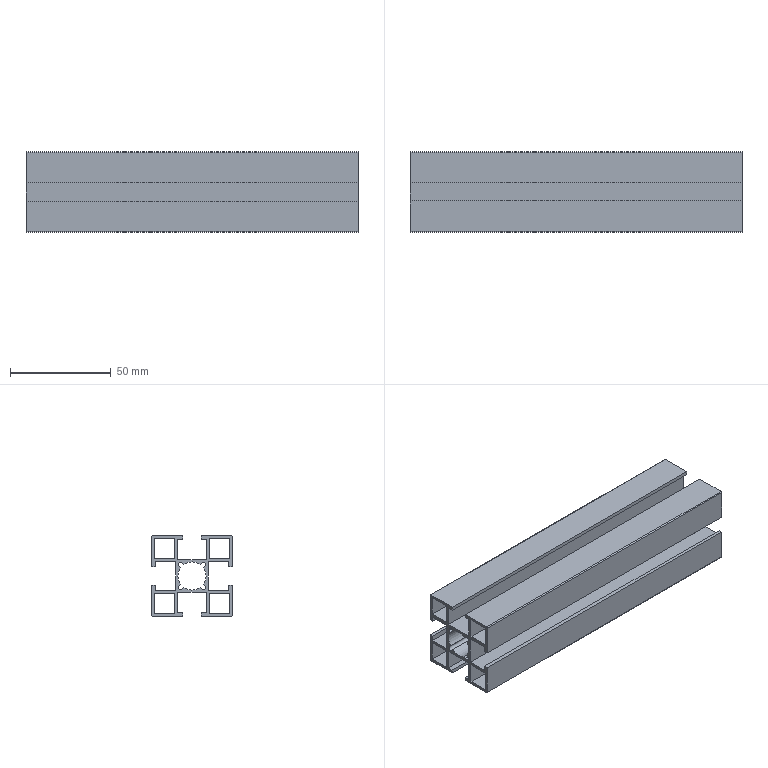Part | 1 solid | 77 faces | box 165 x 40 x 40 mm | volume 65404 mm3 | plane 62 | cylinder 15 | commonest cylinder face diameters 2.2 x6 14 x5 1 x4